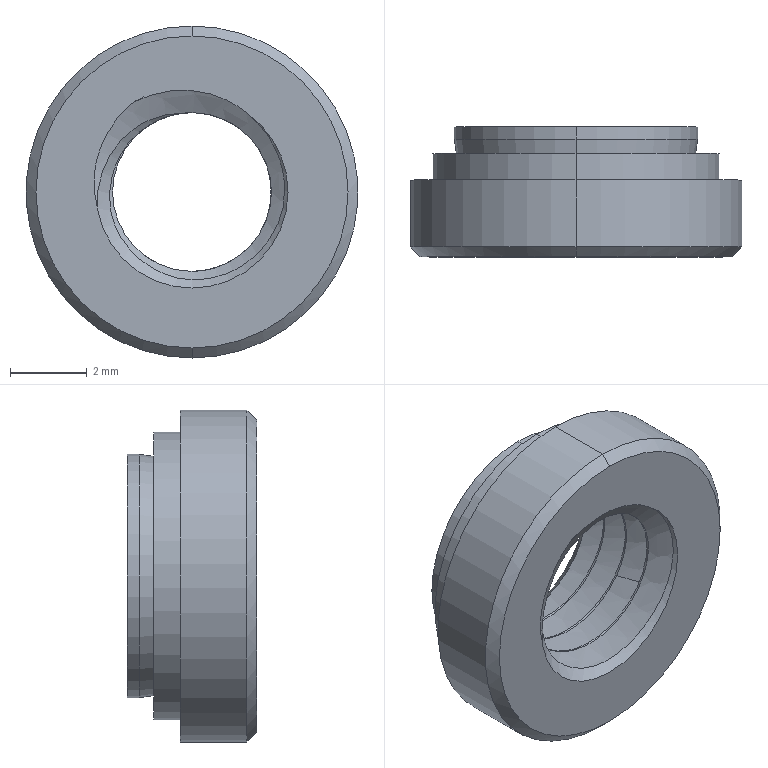Part | NX | features solid 2 | 1 solid | 26 faces | box 8.64 x 3.381 x 8.64 mm | volume 105.585 mm3 | cylinder 12 | cone 6 | plane 4 | spline 4 | commonest cylinder face diameters 4.134 x6 6.33 x2 7.485 x2 8.64 x2